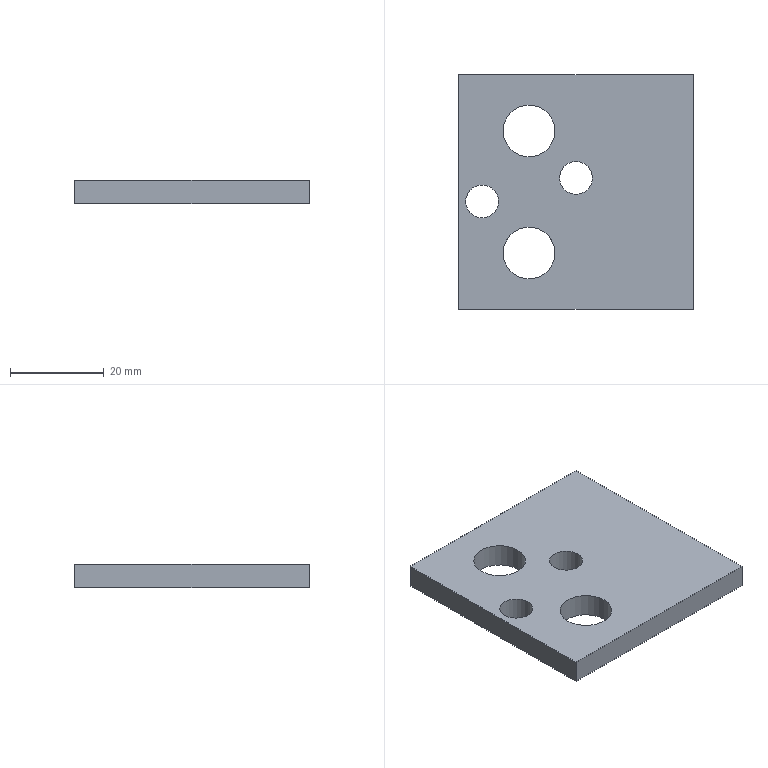Part | NX | features solid 2 | 1 solid | 10 faces | box 50 x 50 x 5 mm | volume 11165 mm3 | plane 6 | cylinder 4 | commonest cylinder face diameters 7 x2 11 x2
STEP:
#1=CARTESIAN_POINT('',(-715.755,-592.,94.));
#2=VERTEX_POINT('',#1);
#3=CARTESIAN_POINT('',(-712.255,-592.,94.));
#4=DIRECTION('',(0.,0.,-1.));
#5=DIRECTION('',(-1.,0.,0.));
#6=AXIS2_PLACEMENT_3D('',#3,#4,#5);
#7=CIRCLE('',#6,3.5);
#8=EDGE_CURVE('',#2,#2,#7,.F.);
#9=ORIENTED_EDGE('',*,*,#8,.T.);
#10=EDGE_LOOP('',(#9));
#11=FACE_BOUND('',#10,.T.);
#12=CARTESIAN_POINT('',(-707.755,-577.,94.));
#13=VERTEX_POINT('',#12);
#14=CARTESIAN_POINT('',(-702.255,-577.,94.));
#15=DIRECTION('',(0.,0.,-1.));
#16=DIRECTION('',(-1.,0.,0.));
#17=AXIS2_PLACEMENT_3D('',#14,#15,#16);
#18=CIRCLE('',#17,5.5);
#19=EDGE_CURVE('',#13,#13,#18,.F.);
#20=ORIENTED_EDGE('',*,*,#19,.T.);
#21=EDGE_LOOP('',(#20));
#22=FACE_BOUND('',#21,.T.);
#23=CARTESIAN_POINT('',(-667.255,-615.,94.));
#24=VERTEX_POINT('',#23);
#25=CARTESIAN_POINT('',(-667.255,-565.,94.));
#26=VERTEX_POINT('',#25);
#27=CARTESIAN_POINT('',(-667.255,-580.049,94.));
#28=DIRECTION('',(0.,1.,0.));
#29=VECTOR('',#28,1000.);
#30=LINE('',#27,#29);
#31=EDGE_CURVE('',#24,#26,#30,.T.);
#32=ORIENTED_EDGE('',*,*,#31,.F.);
#33=CARTESIAN_POINT('',(-717.255,-615.,94.));
#34=VERTEX_POINT('',#33);
#35=CARTESIAN_POINT('',(-687.255,-615.,94.));
#36=DIRECTION('',(-1.,0.,0.));
#37=VECTOR('',#36,1000.);
#38=LINE('',#35,#37);
#39=EDGE_CURVE('',#24,#34,#38,.T.);
#40=ORIENTED_EDGE('',*,*,#39,.T.);
#41=CARTESIAN_POINT('',(-717.255,-565.,94.));
#42=VERTEX_POINT('',#41);
#43=CARTESIAN_POINT('',(-717.255,-580.049,94.));
#44=DIRECTION('',(0.,1.,0.));
#45=VECTOR('',#44,1000.);
#46=LINE('',#43,#45);
#47=EDGE_CURVE('',#34,#42,#46,.T.);
#48=ORIENTED_EDGE('',*,*,#47,.T.);
#49=CARTESIAN_POINT('',(-687.255,-565.,94.));
#50=DIRECTION('',(-1.,0.,0.));
#51=VECTOR('',#50,1000.);
#52=LINE('',#49,#51);
#53=EDGE_CURVE('',#26,#42,#52,.T.);
#54=ORIENTED_EDGE('',*,*,#53,.F.);
#55=EDGE_LOOP('',(#32,#40,#48,#54));
#56=FACE_BOUND('',#55,.T.);
#57=CARTESIAN_POINT('',(-707.755,-603.,94.));
#58=VERTEX_POINT('',#57);
#59=CARTESIAN_POINT('',(-702.255,-603.,94.));
#60=DIRECTION('',(0.,0.,-1.));
#61=DIRECTION('',(-1.,0.,0.));
#62=AXIS2_PLACEMENT_3D('',#59,#60,#61);
#63=CIRCLE('',#62,5.5);
#64=EDGE_CURVE('',#58,#58,#63,.F.);
#65=ORIENTED_EDGE('',*,*,#64,.T.);
#66=EDGE_LOOP('',(#65));
#67=FACE_BOUND('',#66,.T.);
#68=CARTESIAN_POINT('',(-695.755,-587.,94.));
#69=VERTEX_POINT('',#68);
#70=CARTESIAN_POINT('',(-692.255,-587.,94.));
#71=DIRECTION('',(0.,0.,-1.));
#72=DIRECTION('',(-1.,0.,0.));
#73=AXIS2_PLACEMENT_3D('',#70,#71,#72);
#74=CIRCLE('',#73,3.5);
#75=EDGE_CURVE('',#69,#69,#74,.F.);
#76=ORIENTED_EDGE('',*,*,#75,.T.);
#77=EDGE_LOOP('',(#76));
#78=FACE_BOUND('',#77,.T.);
#79=CARTESIAN_POINT('',(-687.255,-580.049,94.));
#80=DIRECTION('',(0.,0.,1.));
#81=DIRECTION('',(1.,0.,0.));
#82=AXIS2_PLACEMENT_3D('',#79,#80,#81);
#83=PLANE('',#82);
#84=ADVANCED_FACE('',(#11,#22,#56,#67,#78),#83,.F.);
#85=CARTESIAN_POINT('',(-715.755,-592.,99.));
#86=VERTEX_POINT('',#85);
#87=CARTESIAN_POINT('',(-712.255,-592.,99.));
#88=DIRECTION('',(0.,0.,-1.));
#89=DIRECTION('',(-1.,0.,0.));
#90=AXIS2_PLACEMENT_3D('',#87,#88,#89);
#91=CIRCLE('',#90,3.5);
#92=EDGE_CURVE('',#86,#86,#91,.F.);
#93=ORIENTED_EDGE('',*,*,#92,.F.);
#94=EDGE_LOOP('',(#93));
#95=FACE_BOUND('',#94,.T.);
#96=CARTESIAN_POINT('',(-707.755,-577.,99.));
#97=VERTEX_POINT('',#96);
#98=CARTESIAN_POINT('',(-702.255,-577.,99.));
#99=DIRECTION('',(0.,0.,-1.));
#100=DIRECTION('',(-1.,0.,0.));
#101=AXIS2_PLACEMENT_3D('',#98,#99,#100);
#102=CIRCLE('',#101,5.5);
#103=EDGE_CURVE('',#97,#97,#102,.F.);
#104=ORIENTED_EDGE('',*,*,#103,.F.);
#105=EDGE_LOOP('',(#104));
#106=FACE_BOUND('',#105,.T.);
#107=CARTESIAN_POINT('',(-667.255,-615.,99.));
#108=VERTEX_POINT('',#107);
#109=CARTESIAN_POINT('',(-667.255,-565.,99.));
#110=VERTEX_POINT('',#109);
#111=CARTESIAN_POINT('',(-667.255,-580.049,99.));
#112=DIRECTION('',(0.,1.,0.));
#113=VECTOR('',#112,1000.);
#114=LINE('',#111,#113);
#115=EDGE_CURVE('',#108,#110,#114,.T.);
#116=ORIENTED_EDGE('',*,*,#115,.T.);
#117=CARTESIAN_POINT('',(-717.255,-565.,99.));
#118=VERTEX_POINT('',#117);
#119=CARTESIAN_POINT('',(-687.255,-565.,99.));
#120=DIRECTION('',(-1.,0.,0.));
#121=VECTOR('',#120,1000.);
#122=LINE('',#119,#121);
#123=EDGE_CURVE('',#110,#118,#122,.T.);
#124=ORIENTED_EDGE('',*,*,#123,.T.);
#125=CARTESIAN_POINT('',(-717.255,-615.,99.));
#126=VERTEX_POINT('',#125);
#127=CARTESIAN_POINT('',(-717.255,-580.049,99.));
#128=DIRECTION('',(0.,1.,0.));
#129=VECTOR('',#128,1000.);
#130=LINE('',#127,#129);
#131=EDGE_CURVE('',#126,#118,#130,.T.);
#132=ORIENTED_EDGE('',*,*,#131,.F.);
#133=CARTESIAN_POINT('',(-687.255,-615.,99.));
#134=DIRECTION('',(-1.,0.,0.));
#135=VECTOR('',#134,1000.);
#136=LINE('',#133,#135);
#137=EDGE_CURVE('',#108,#126,#136,.T.);
#138=ORIENTED_EDGE('',*,*,#137,.F.);
#139=EDGE_LOOP('',(#116,#124,#132,#138));
#140=FACE_BOUND('',#139,.T.);
#141=CARTESIAN_POINT('',(-707.755,-603.,99.));
#142=VERTEX_POINT('',#141);
#143=CARTESIAN_POINT('',(-702.255,-603.,99.));
#144=DIRECTION('',(0.,0.,-1.));
#145=DIRECTION('',(-1.,0.,0.));
#146=AXIS2_PLACEMENT_3D('',#143,#144,#145);
#147=CIRCLE('',#146,5.5);
#148=EDGE_CURVE('',#142,#142,#147,.F.);
#149=ORIENTED_EDGE('',*,*,#148,.F.);
#150=EDGE_LOOP('',(#149));
#151=FACE_BOUND('',#150,.T.);
#152=CARTESIAN_POINT('',(-695.755,-587.,99.));
#153=VERTEX_POINT('',#152);
#154=CARTESIAN_POINT('',(-692.255,-587.,99.));
#155=DIRECTION('',(0.,0.,-1.));
#156=DIRECTION('',(-1.,0.,0.));
#157=AXIS2_PLACEMENT_3D('',#154,#155,#156);
#158=CIRCLE('',#157,3.5);
#159=EDGE_CURVE('',#153,#153,#158,.F.);
#160=ORIENTED_EDGE('',*,*,#159,.F.);
#161=EDGE_LOOP('',(#160));
#162=FACE_BOUND('',#161,.T.);
#163=CARTESIAN_POINT('',(-687.255,-580.049,99.));
#164=DIRECTION('',(0.,0.,1.));
#165=DIRECTION('',(1.,0.,0.));
#166=AXIS2_PLACEMENT_3D('',#163,#164,#165);
#167=PLANE('',#166);
#168=ADVANCED_FACE('',(#95,#106,#140,#151,#162),#167,.T.);
#169=ORIENTED_EDGE('',*,*,#115,.F.);
#170=CARTESIAN_POINT('',(-667.255,-615.,64.));
#171=DIRECTION('',(0.,0.,1.));
#172=VECTOR('',#171,1000.);
#173=LINE('',#170,#172);
#174=EDGE_CURVE('',#24,#108,#173,.T.);
#175=ORIENTED_EDGE('',*,*,#174,.F.);
#176=ORIENTED_EDGE('',*,*,#31,.T.);
#177=CARTESIAN_POINT('',(-667.255,-565.,64.));
#178=DIRECTION('',(0.,0.,1.));
#179=VECTOR('',#178,1000.);
#180=LINE('',#177,#179);
#181=EDGE_CURVE('',#26,#110,#180,.T.);
#182=ORIENTED_EDGE('',*,*,#181,.T.);
#183=EDGE_LOOP('',(#169,#175,#176,#182));
#184=FACE_BOUND('',#183,.T.);
#185=CARTESIAN_POINT('',(-667.255,-584.713,64.));
#186=DIRECTION('',(1.,0.,0.));
#187=DIRECTION('',(0.,0.,-1.));
#188=AXIS2_PLACEMENT_3D('',#185,#186,#187);
#189=PLANE('',#188);
#190=ADVANCED_FACE('',(#184),#189,.T.);
#191=ORIENTED_EDGE('',*,*,#123,.F.);
#192=ORIENTED_EDGE('',*,*,#181,.F.);
#193=ORIENTED_EDGE('',*,*,#53,.T.);
#194=CARTESIAN_POINT('',(-717.255,-565.,94.));
#195=DIRECTION('',(0.,0.,1.));
#196=VECTOR('',#195,1000.);
#197=LINE('',#194,#196);
#198=EDGE_CURVE('',#42,#118,#197,.T.);
#199=ORIENTED_EDGE('',*,*,#198,.T.);
#200=EDGE_LOOP('',(#191,#192,#193,#199));
#201=FACE_BOUND('',#200,.T.);
#202=CARTESIAN_POINT('',(-687.255,-565.,94.));
#203=DIRECTION('',(0.,1.,0.));
#204=DIRECTION('',(0.,0.,1.));
#205=AXIS2_PLACEMENT_3D('',#202,#203,#204);
#206=PLANE('',#205);
#207=ADVANCED_FACE('',(#201),#206,.T.);
#208=ORIENTED_EDGE('',*,*,#131,.T.);
#209=ORIENTED_EDGE('',*,*,#198,.F.);
#210=ORIENTED_EDGE('',*,*,#47,.F.);
#211=CARTESIAN_POINT('',(-717.255,-615.,94.));
#212=DIRECTION('',(0.,0.,1.));
#213=VECTOR('',#212,1000.);
#214=LINE('',#211,#213);
#215=EDGE_CURVE('',#34,#126,#214,.T.);
#216=ORIENTED_EDGE('',*,*,#215,.T.);
#217=EDGE_LOOP('',(#208,#209,#210,#216));
#218=FACE_BOUND('',#217,.T.);
#219=CARTESIAN_POINT('',(-717.255,-580.049,94.));
#220=DIRECTION('',(1.,0.,0.));
#221=DIRECTION('',(0.,0.,-1.));
#222=AXIS2_PLACEMENT_3D('',#219,#220,#221);
#223=PLANE('',#222);
#224=ADVANCED_FACE('',(#218),#223,.F.);
#225=ORIENTED_EDGE('',*,*,#137,.T.);
#226=ORIENTED_EDGE('',*,*,#215,.F.);
#227=ORIENTED_EDGE('',*,*,#39,.F.);
#228=ORIENTED_EDGE('',*,*,#174,.T.);
#229=EDGE_LOOP('',(#225,#226,#227,#228));
#230=FACE_BOUND('',#229,.T.);
#231=CARTESIAN_POINT('',(-687.255,-615.,94.));
#232=DIRECTION('',(0.,1.,0.));
#233=DIRECTION('',(0.,0.,1.));
#234=AXIS2_PLACEMENT_3D('',#231,#232,#233);
#235=PLANE('',#234);
#236=ADVANCED_FACE('',(#230),#235,.F.);
#237=ORIENTED_EDGE('',*,*,#103,.T.);
#238=EDGE_LOOP('',(#237));
#239=FACE_BOUND('',#238,.T.);
#240=ORIENTED_EDGE('',*,*,#19,.F.);
#241=EDGE_LOOP('',(#240));
#242=FACE_BOUND('',#241,.T.);
#243=CARTESIAN_POINT('',(-702.255,-577.,44.));
#244=DIRECTION('',(0.,0.,1.));
#245=DIRECTION('',(-1.,0.,0.));
#246=AXIS2_PLACEMENT_3D('',#243,#244,#245);
#247=CYLINDRICAL_SURFACE('',#246,5.5);
#248=ADVANCED_FACE('',(#239,#242),#247,.F.);
#249=ORIENTED_EDGE('',*,*,#148,.T.);
#250=EDGE_LOOP('',(#249));
#251=FACE_BOUND('',#250,.T.);
#252=ORIENTED_EDGE('',*,*,#64,.F.);
#253=EDGE_LOOP('',(#252));
#254=FACE_BOUND('',#253,.T.);
#255=CARTESIAN_POINT('',(-702.255,-603.,44.));
#256=DIRECTION('',(0.,0.,1.));
#257=DIRECTION('',(-1.,0.,0.));
#258=AXIS2_PLACEMENT_3D('',#255,#256,#257);
#259=CYLINDRICAL_SURFACE('',#258,5.5);
#260=ADVANCED_FACE('',(#251,#254),#259,.F.);
#261=ORIENTED_EDGE('',*,*,#92,.T.);
#262=EDGE_LOOP('',(#261));
#263=FACE_BOUND('',#262,.T.);
#264=ORIENTED_EDGE('',*,*,#8,.F.);
#265=EDGE_LOOP('',(#264));
#266=FACE_BOUND('',#265,.T.);
#267=CARTESIAN_POINT('',(-712.255,-592.,44.));
#268=DIRECTION('',(0.,0.,1.));
#269=DIRECTION('',(-1.,0.,0.));
#270=AXIS2_PLACEMENT_3D('',#267,#268,#269);
#271=CYLINDRICAL_SURFACE('',#270,3.5);
#272=ADVANCED_FACE('',(#263,#266),#271,.F.);
#273=ORIENTED_EDGE('',*,*,#159,.T.);
#274=EDGE_LOOP('',(#273));
#275=FACE_BOUND('',#274,.T.);
#276=ORIENTED_EDGE('',*,*,#75,.F.);
#277=EDGE_LOOP('',(#276));
#278=FACE_BOUND('',#277,.T.);
#279=CARTESIAN_POINT('',(-692.255,-587.,44.));
#280=DIRECTION('',(0.,0.,1.));
#281=DIRECTION('',(-1.,0.,0.));
#282=AXIS2_PLACEMENT_3D('',#279,#280,#281);
#283=CYLINDRICAL_SURFACE('',#282,3.5);
#284=ADVANCED_FACE('',(#275,#278),#283,.F.);
#285=CLOSED_SHELL('',(#84,#168,#190,#207,#224,#236,#248,#260,#272,#284));
#286=MANIFOLD_SOLID_BREP('',#285);
#287=(LENGTH_UNIT()NAMED_UNIT(*)SI_UNIT(.MILLI.,.METRE.));
#288=UNCERTAINTY_MEASURE_WITH_UNIT(LENGTH_MEASURE(0.00001),#287,'','');
#289=(NAMED_UNIT(*)PLANE_ANGLE_UNIT()SI_UNIT($,.RADIAN.));
#290=(NAMED_UNIT(*)SI_UNIT($,.STERADIAN.)SOLID_ANGLE_UNIT());
#291=(GEOMETRIC_REPRESENTATION_CONTEXT(3)GLOBAL_UNCERTAINTY_ASSIGNED_CONTEXT((#288))GLOBAL_UNIT_ASSIGNED_CONTEXT((#287,#289,#290))REPRESENTATION_CONTEXT('',''));
#292=ADVANCED_BREP_SHAPE_REPRESENTATION('',(#286),#291);